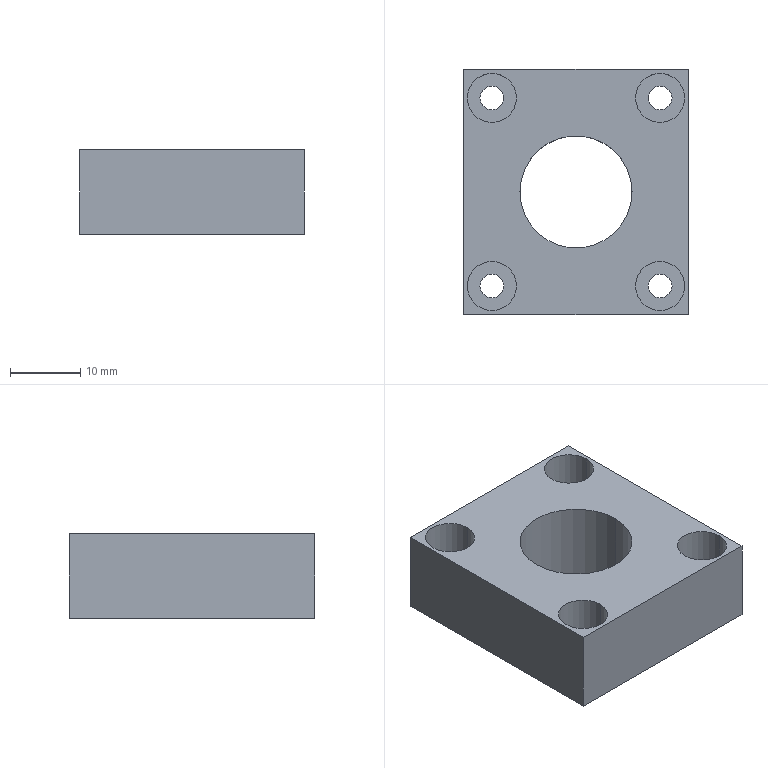Part | NX | features BREP 1 | 1 solid | 28 faces | box 32 x 35 x 12 mm | volume 10003 mm3 | cylinder 18 | plane 10 | commonest cylinder face diameters 3.4 x8 7 x8 16 x2
STEP:
#1=CARTESIAN_POINT('',(8.5,-13.416,12.));
#2=VERTEX_POINT('',#1);
#3=CARTESIAN_POINT('',(8.5,-13.416,7.));
#4=VERTEX_POINT('',#3);
#5=CARTESIAN_POINT('',(8.5,-13.416,12.));
#6=DIRECTION('',(0.,0.,1.));
#7=VECTOR('',#6,1000.);
#8=LINE('',#5,#7);
#9=EDGE_CURVE('',#2,#4,#8,.F.);
#10=ORIENTED_EDGE('',*,*,#9,.T.);
#11=CARTESIAN_POINT('',(15.5,-13.416,7.));
#12=VERTEX_POINT('',#11);
#13=CARTESIAN_POINT('',(12.,-13.416,7.));
#14=DIRECTION('',(0.,0.,1.));
#15=DIRECTION('',(1.,0.,0.));
#16=AXIS2_PLACEMENT_3D('',#13,#14,#15);
#17=CIRCLE('',#16,3.5);
#18=EDGE_CURVE('',#12,#4,#17,.T.);
#19=ORIENTED_EDGE('',*,*,#18,.F.);
#20=CARTESIAN_POINT('',(15.5,-13.416,12.));
#21=VERTEX_POINT('',#20);
#22=CARTESIAN_POINT('',(15.5,-13.416,12.));
#23=DIRECTION('',(0.,0.,1.));
#24=VECTOR('',#23,1000.);
#25=LINE('',#22,#24);
#26=EDGE_CURVE('',#21,#12,#25,.F.);
#27=ORIENTED_EDGE('',*,*,#26,.F.);
#28=CARTESIAN_POINT('',(12.,-13.416,12.));
#29=DIRECTION('',(0.,0.,1.));
#30=DIRECTION('',(1.,0.,0.));
#31=AXIS2_PLACEMENT_3D('',#28,#29,#30);
#32=CIRCLE('',#31,3.5);
#33=EDGE_CURVE('',#21,#2,#32,.T.);
#34=ORIENTED_EDGE('',*,*,#33,.T.);
#35=EDGE_LOOP('',(#10,#19,#27,#34));
#36=FACE_BOUND('',#35,.T.);
#37=CARTESIAN_POINT('',(12.,-13.416,12.));
#38=DIRECTION('',(0.,0.,1.));
#39=DIRECTION('',(1.,0.,0.));
#40=AXIS2_PLACEMENT_3D('',#37,#38,#39);
#41=CYLINDRICAL_SURFACE('',#40,3.5);
#42=ADVANCED_FACE('',(#36),#41,.F.);
#43=ORIENTED_EDGE('',*,*,#18,.T.);
#44=CARTESIAN_POINT('',(12.,-13.416,7.));
#45=DIRECTION('',(0.,0.,1.));
#46=DIRECTION('',(1.,0.,0.));
#47=AXIS2_PLACEMENT_3D('',#44,#45,#46);
#48=CIRCLE('',#47,3.5);
#49=EDGE_CURVE('',#4,#12,#48,.T.);
#50=ORIENTED_EDGE('',*,*,#49,.T.);
#51=EDGE_LOOP('',(#43,#50));
#52=FACE_BOUND('',#51,.T.);
#53=CARTESIAN_POINT('',(13.7,-13.416,7.));
#54=VERTEX_POINT('',#53);
#55=CARTESIAN_POINT('',(10.3,-13.416,7.));
#56=VERTEX_POINT('',#55);
#57=CARTESIAN_POINT('',(12.,-13.416,7.));
#58=DIRECTION('',(0.,0.,1.));
#59=DIRECTION('',(1.,0.,0.));
#60=AXIS2_PLACEMENT_3D('',#57,#58,#59);
#61=CIRCLE('',#60,1.7);
#62=EDGE_CURVE('',#54,#56,#61,.T.);
#63=ORIENTED_EDGE('',*,*,#62,.F.);
#64=CARTESIAN_POINT('',(12.,-13.416,7.));
#65=DIRECTION('',(0.,0.,1.));
#66=DIRECTION('',(1.,0.,0.));
#67=AXIS2_PLACEMENT_3D('',#64,#65,#66);
#68=CIRCLE('',#67,1.7);
#69=EDGE_CURVE('',#56,#54,#68,.T.);
#70=ORIENTED_EDGE('',*,*,#69,.F.);
#71=EDGE_LOOP('',(#63,#70));
#72=FACE_BOUND('',#71,.T.);
#73=CARTESIAN_POINT('',(13.7,-13.416,7.));
#74=DIRECTION('',(0.,0.,-1.));
#75=DIRECTION('',(-1.,0.,0.));
#76=AXIS2_PLACEMENT_3D('',#73,#74,#75);
#77=PLANE('',#76);
#78=ADVANCED_FACE('',(#52,#72),#77,.F.);
#79=CARTESIAN_POINT('',(10.3,-13.416,0.));
#80=VERTEX_POINT('',#79);
#81=CARTESIAN_POINT('',(10.3,-13.416,12.));
#82=DIRECTION('',(0.,0.,1.));
#83=VECTOR('',#82,1000.);
#84=LINE('',#81,#83);
#85=EDGE_CURVE('',#56,#80,#84,.F.);
#86=ORIENTED_EDGE('',*,*,#85,.T.);
#87=CARTESIAN_POINT('',(13.7,-13.416,0.));
#88=VERTEX_POINT('',#87);
#89=CARTESIAN_POINT('',(12.,-13.416,0.));
#90=DIRECTION('',(0.,0.,1.));
#91=DIRECTION('',(1.,0.,0.));
#92=AXIS2_PLACEMENT_3D('',#89,#90,#91);
#93=CIRCLE('',#92,1.7);
#94=EDGE_CURVE('',#88,#80,#93,.T.);
#95=ORIENTED_EDGE('',*,*,#94,.F.);
#96=CARTESIAN_POINT('',(13.7,-13.416,12.));
#97=DIRECTION('',(0.,0.,1.));
#98=VECTOR('',#97,1000.);
#99=LINE('',#96,#98);
#100=EDGE_CURVE('',#54,#88,#99,.F.);
#101=ORIENTED_EDGE('',*,*,#100,.F.);
#102=ORIENTED_EDGE('',*,*,#62,.T.);
#103=EDGE_LOOP('',(#86,#95,#101,#102));
#104=FACE_BOUND('',#103,.T.);
#105=CARTESIAN_POINT('',(12.,-13.416,12.));
#106=DIRECTION('',(0.,0.,1.));
#107=DIRECTION('',(1.,0.,0.));
#108=AXIS2_PLACEMENT_3D('',#105,#106,#107);
#109=CYLINDRICAL_SURFACE('',#108,1.7);
#110=ADVANCED_FACE('',(#104),#109,.F.);
#111=CARTESIAN_POINT('',(-15.5,-13.416,12.));
#112=VERTEX_POINT('',#111);
#113=CARTESIAN_POINT('',(-15.5,-13.416,7.));
#114=VERTEX_POINT('',#113);
#115=CARTESIAN_POINT('',(-15.5,-13.416,12.));
#116=DIRECTION('',(0.,0.,1.));
#117=VECTOR('',#116,1000.);
#118=LINE('',#115,#117);
#119=EDGE_CURVE('',#112,#114,#118,.F.);
#120=ORIENTED_EDGE('',*,*,#119,.T.);
#121=CARTESIAN_POINT('',(-8.5,-13.416,7.));
#122=VERTEX_POINT('',#121);
#123=CARTESIAN_POINT('',(-12.,-13.416,7.));
#124=DIRECTION('',(0.,0.,1.));
#125=DIRECTION('',(1.,0.,0.));
#126=AXIS2_PLACEMENT_3D('',#123,#124,#125);
#127=CIRCLE('',#126,3.5);
#128=EDGE_CURVE('',#122,#114,#127,.T.);
#129=ORIENTED_EDGE('',*,*,#128,.F.);
#130=CARTESIAN_POINT('',(-8.5,-13.416,12.));
#131=VERTEX_POINT('',#130);
#132=CARTESIAN_POINT('',(-8.5,-13.416,12.));
#133=DIRECTION('',(0.,0.,1.));
#134=VECTOR('',#133,1000.);
#135=LINE('',#132,#134);
#136=EDGE_CURVE('',#131,#122,#135,.F.);
#137=ORIENTED_EDGE('',*,*,#136,.F.);
#138=CARTESIAN_POINT('',(-12.,-13.416,12.));
#139=DIRECTION('',(0.,0.,1.));
#140=DIRECTION('',(1.,0.,0.));
#141=AXIS2_PLACEMENT_3D('',#138,#139,#140);
#142=CIRCLE('',#141,3.5);
#143=EDGE_CURVE('',#131,#112,#142,.T.);
#144=ORIENTED_EDGE('',*,*,#143,.T.);
#145=EDGE_LOOP('',(#120,#129,#137,#144));
#146=FACE_BOUND('',#145,.T.);
#147=CARTESIAN_POINT('',(-12.,-13.416,12.));
#148=DIRECTION('',(0.,0.,1.));
#149=DIRECTION('',(1.,0.,0.));
#150=AXIS2_PLACEMENT_3D('',#147,#148,#149);
#151=CYLINDRICAL_SURFACE('',#150,3.5);
#152=ADVANCED_FACE('',(#146),#151,.F.);
#153=ORIENTED_EDGE('',*,*,#128,.T.);
#154=CARTESIAN_POINT('',(-12.,-13.416,7.));
#155=DIRECTION('',(0.,0.,1.));
#156=DIRECTION('',(1.,0.,0.));
#157=AXIS2_PLACEMENT_3D('',#154,#155,#156);
#158=CIRCLE('',#157,3.5);
#159=EDGE_CURVE('',#114,#122,#158,.T.);
#160=ORIENTED_EDGE('',*,*,#159,.T.);
#161=EDGE_LOOP('',(#153,#160));
#162=FACE_BOUND('',#161,.T.);
#163=CARTESIAN_POINT('',(-10.3,-13.416,7.));
#164=VERTEX_POINT('',#163);
#165=CARTESIAN_POINT('',(-13.7,-13.416,7.));
#166=VERTEX_POINT('',#165);
#167=CARTESIAN_POINT('',(-12.,-13.416,7.));
#168=DIRECTION('',(0.,0.,1.));
#169=DIRECTION('',(1.,0.,0.));
#170=AXIS2_PLACEMENT_3D('',#167,#168,#169);
#171=CIRCLE('',#170,1.7);
#172=EDGE_CURVE('',#164,#166,#171,.T.);
#173=ORIENTED_EDGE('',*,*,#172,.F.);
#174=CARTESIAN_POINT('',(-12.,-13.416,7.));
#175=DIRECTION('',(0.,0.,1.));
#176=DIRECTION('',(1.,0.,0.));
#177=AXIS2_PLACEMENT_3D('',#174,#175,#176);
#178=CIRCLE('',#177,1.7);
#179=EDGE_CURVE('',#166,#164,#178,.T.);
#180=ORIENTED_EDGE('',*,*,#179,.F.);
#181=EDGE_LOOP('',(#173,#180));
#182=FACE_BOUND('',#181,.T.);
#183=CARTESIAN_POINT('',(-10.3,-13.416,7.));
#184=DIRECTION('',(0.,0.,-1.));
#185=DIRECTION('',(-1.,0.,0.));
#186=AXIS2_PLACEMENT_3D('',#183,#184,#185);
#187=PLANE('',#186);
#188=ADVANCED_FACE('',(#162,#182),#187,.F.);
#189=CARTESIAN_POINT('',(-13.7,-13.416,0.));
#190=VERTEX_POINT('',#189);
#191=CARTESIAN_POINT('',(-13.7,-13.416,12.));
#192=DIRECTION('',(0.,0.,1.));
#193=VECTOR('',#192,1000.);
#194=LINE('',#191,#193);
#195=EDGE_CURVE('',#166,#190,#194,.F.);
#196=ORIENTED_EDGE('',*,*,#195,.T.);
#197=CARTESIAN_POINT('',(-10.3,-13.416,0.));
#198=VERTEX_POINT('',#197);
#199=CARTESIAN_POINT('',(-12.,-13.416,0.));
#200=DIRECTION('',(0.,0.,1.));
#201=DIRECTION('',(1.,0.,0.));
#202=AXIS2_PLACEMENT_3D('',#199,#200,#201);
#203=CIRCLE('',#202,1.7);
#204=EDGE_CURVE('',#198,#190,#203,.T.);
#205=ORIENTED_EDGE('',*,*,#204,.F.);
#206=CARTESIAN_POINT('',(-10.3,-13.416,12.));
#207=DIRECTION('',(0.,0.,1.));
#208=VECTOR('',#207,1000.);
#209=LINE('',#206,#208);
#210=EDGE_CURVE('',#164,#198,#209,.F.);
#211=ORIENTED_EDGE('',*,*,#210,.F.);
#212=ORIENTED_EDGE('',*,*,#172,.T.);
#213=EDGE_LOOP('',(#196,#205,#211,#212));
#214=FACE_BOUND('',#213,.T.);
#215=CARTESIAN_POINT('',(-12.,-13.416,12.));
#216=DIRECTION('',(0.,0.,1.));
#217=DIRECTION('',(1.,0.,0.));
#218=AXIS2_PLACEMENT_3D('',#215,#216,#217);
#219=CYLINDRICAL_SURFACE('',#218,1.7);
#220=ADVANCED_FACE('',(#214),#219,.F.);
#221=CARTESIAN_POINT('',(8.5,13.416,12.));
#222=VERTEX_POINT('',#221);
#223=CARTESIAN_POINT('',(8.5,13.416,7.));
#224=VERTEX_POINT('',#223);
#225=CARTESIAN_POINT('',(8.5,13.416,12.));
#226=DIRECTION('',(0.,0.,1.));
#227=VECTOR('',#226,1000.);
#228=LINE('',#225,#227);
#229=EDGE_CURVE('',#222,#224,#228,.F.);
#230=ORIENTED_EDGE('',*,*,#229,.T.);
#231=CARTESIAN_POINT('',(15.5,13.416,7.));
#232=VERTEX_POINT('',#231);
#233=CARTESIAN_POINT('',(12.,13.416,7.));
#234=DIRECTION('',(0.,0.,1.));
#235=DIRECTION('',(1.,0.,0.));
#236=AXIS2_PLACEMENT_3D('',#233,#234,#235);
#237=CIRCLE('',#236,3.5);
#238=EDGE_CURVE('',#232,#224,#237,.T.);
#239=ORIENTED_EDGE('',*,*,#238,.F.);
#240=CARTESIAN_POINT('',(15.5,13.416,12.));
#241=VERTEX_POINT('',#240);
#242=CARTESIAN_POINT('',(15.5,13.416,12.));
#243=DIRECTION('',(0.,0.,1.));
#244=VECTOR('',#243,1000.);
#245=LINE('',#242,#244);
#246=EDGE_CURVE('',#241,#232,#245,.F.);
#247=ORIENTED_EDGE('',*,*,#246,.F.);
#248=CARTESIAN_POINT('',(12.,13.416,12.));
#249=DIRECTION('',(0.,0.,1.));
#250=DIRECTION('',(1.,0.,0.));
#251=AXIS2_PLACEMENT_3D('',#248,#249,#250);
#252=CIRCLE('',#251,3.5);
#253=EDGE_CURVE('',#241,#222,#252,.T.);
#254=ORIENTED_EDGE('',*,*,#253,.T.);
#255=EDGE_LOOP('',(#230,#239,#247,#254));
#256=FACE_BOUND('',#255,.T.);
#257=CARTESIAN_POINT('',(12.,13.416,12.));
#258=DIRECTION('',(0.,0.,1.));
#259=DIRECTION('',(1.,0.,0.));
#260=AXIS2_PLACEMENT_3D('',#257,#258,#259);
#261=CYLINDRICAL_SURFACE('',#260,3.5);
#262=ADVANCED_FACE('',(#256),#261,.F.);
#263=ORIENTED_EDGE('',*,*,#238,.T.);
#264=CARTESIAN_POINT('',(12.,13.416,7.));
#265=DIRECTION('',(0.,0.,1.));
#266=DIRECTION('',(1.,0.,0.));
#267=AXIS2_PLACEMENT_3D('',#264,#265,#266);
#268=CIRCLE('',#267,3.5);
#269=EDGE_CURVE('',#224,#232,#268,.T.);
#270=ORIENTED_EDGE('',*,*,#269,.T.);
#271=EDGE_LOOP('',(#263,#270));
#272=FACE_BOUND('',#271,.T.);
#273=CARTESIAN_POINT('',(13.7,13.416,7.));
#274=VERTEX_POINT('',#273);
#275=CARTESIAN_POINT('',(10.3,13.416,7.));
#276=VERTEX_POINT('',#275);
#277=CARTESIAN_POINT('',(12.,13.416,7.));
#278=DIRECTION('',(0.,0.,1.));
#279=DIRECTION('',(1.,0.,0.));
#280=AXIS2_PLACEMENT_3D('',#277,#278,#279);
#281=CIRCLE('',#280,1.7);
#282=EDGE_CURVE('',#274,#276,#281,.T.);
#283=ORIENTED_EDGE('',*,*,#282,.F.);
#284=CARTESIAN_POINT('',(12.,13.416,7.));
#285=DIRECTION('',(0.,0.,1.));
#286=DIRECTION('',(1.,0.,0.));
#287=AXIS2_PLACEMENT_3D('',#284,#285,#286);
#288=CIRCLE('',#287,1.7);
#289=EDGE_CURVE('',#276,#274,#288,.T.);
#290=ORIENTED_EDGE('',*,*,#289,.F.);
#291=EDGE_LOOP('',(#283,#290));
#292=FACE_BOUND('',#291,.T.);
#293=CARTESIAN_POINT('',(13.7,13.416,7.));
#294=DIRECTION('',(0.,0.,-1.));
#295=DIRECTION('',(-1.,0.,0.));
#296=AXIS2_PLACEMENT_3D('',#293,#294,#295);
#297=PLANE('',#296);
#298=ADVANCED_FACE('',(#272,#292),#297,.F.);
#299=CARTESIAN_POINT('',(10.3,13.416,0.));
#300=VERTEX_POINT('',#299);
#301=CARTESIAN_POINT('',(10.3,13.416,12.));
#302=DIRECTION('',(0.,0.,1.));
#303=VECTOR('',#302,1000.);
#304=LINE('',#301,#303);
#305=EDGE_CURVE('',#276,#300,#304,.F.);
#306=ORIENTED_EDGE('',*,*,#305,.T.);
#307=CARTESIAN_POINT('',(13.7,13.416,0.));
#308=VERTEX_POINT('',#307);
#309=CARTESIAN_POINT('',(12.,13.416,0.));
#310=DIRECTION('',(0.,0.,1.));
#311=DIRECTION('',(1.,0.,0.));
#312=AXIS2_PLACEMENT_3D('',#309,#310,#311);
#313=CIRCLE('',#312,1.7);
#314=EDGE_CURVE('',#308,#300,#313,.T.);
#315=ORIENTED_EDGE('',*,*,#314,.F.);
#316=CARTESIAN_POINT('',(13.7,13.416,12.));
#317=DIRECTION('',(0.,0.,1.));
#318=VECTOR('',#317,1000.);
#319=LINE('',#316,#318);
#320=EDGE_CURVE('',#274,#308,#319,.F.);
#321=ORIENTED_EDGE('',*,*,#320,.F.);
#322=ORIENTED_EDGE('',*,*,#282,.T.);
#323=EDGE_LOOP('',(#306,#315,#321,#322));
#324=FACE_BOUND('',#323,.T.);
#325=CARTESIAN_POINT('',(12.,13.416,12.));
#326=DIRECTION('',(0.,0.,1.));
#327=DIRECTION('',(1.,0.,0.));
#328=AXIS2_PLACEMENT_3D('',#325,#326,#327);
#329=CYLINDRICAL_SURFACE('',#328,1.7);
#330=ADVANCED_FACE('',(#324),#329,.F.);
#331=CARTESIAN_POINT('',(-15.5,13.416,12.));
#332=VERTEX_POINT('',#331);
#333=CARTESIAN_POINT('',(-15.5,13.416,7.));
#334=VERTEX_POINT('',#333);
#335=CARTESIAN_POINT('',(-15.5,13.416,12.));
#336=DIRECTION('',(0.,0.,1.));
#337=VECTOR('',#336,1000.);
#338=LINE('',#335,#337);
#339=EDGE_CURVE('',#332,#334,#338,.F.);
#340=ORIENTED_EDGE('',*,*,#339,.T.);
#341=CARTESIAN_POINT('',(-8.5,13.416,7.));
#342=VERTEX_POINT('',#341);
#343=CARTESIAN_POINT('',(-12.,13.416,7.));
#344=DIRECTION('',(0.,0.,1.));
#345=DIRECTION('',(1.,0.,0.));
#346=AXIS2_PLACEMENT_3D('',#343,#344,#345);
#347=CIRCLE('',#346,3.5);
#348=EDGE_CURVE('',#342,#334,#347,.T.);
#349=ORIENTED_EDGE('',*,*,#348,.F.);
#350=CARTESIAN_POINT('',(-8.5,13.416,12.));
#351=VERTEX_POINT('',#350);
#352=CARTESIAN_POINT('',(-8.5,13.416,12.));
#353=DIRECTION('',(0.,0.,1.));
#354=VECTOR('',#353,1000.);
#355=LINE('',#352,#354);
#356=EDGE_CURVE('',#351,#342,#355,.F.);
#357=ORIENTED_EDGE('',*,*,#356,.F.);
#358=CARTESIAN_POINT('',(-12.,13.416,12.));
#359=DIRECTION('',(0.,0.,1.));
#360=DIRECTION('',(1.,0.,0.));
#361=AXIS2_PLACEMENT_3D('',#358,#359,#360);
#362=CIRCLE('',#361,3.5);
#363=EDGE_CURVE('',#351,#332,#362,.T.);
#364=ORIENTED_EDGE('',*,*,#363,.T.);
#365=EDGE_LOOP('',(#340,#349,#357,#364));
#366=FACE_BOUND('',#365,.T.);
#367=CARTESIAN_POINT('',(-12.,13.416,12.));
#368=DIRECTION('',(0.,0.,1.));
#369=DIRECTION('',(1.,0.,0.));
#370=AXIS2_PLACEMENT_3D('',#367,#368,#369);
#371=CYLINDRICAL_SURFACE('',#370,3.5);
#372=ADVANCED_FACE('',(#366),#371,.F.);
#373=ORIENTED_EDGE('',*,*,#348,.T.);
#374=CARTESIAN_POINT('',(-12.,13.416,7.));
#375=DIRECTION('',(0.,0.,1.));
#376=DIRECTION('',(1.,0.,0.));
#377=AXIS2_PLACEMENT_3D('',#374,#375,#376);
#378=CIRCLE('',#377,3.5);
#379=EDGE_CURVE('',#334,#342,#378,.T.);
#380=ORIENTED_EDGE('',*,*,#379,.T.);
#381=EDGE_LOOP('',(#373,#380));
#382=FACE_BOUND('',#381,.T.);
#383=CARTESIAN_POINT('',(-10.3,13.416,7.));
#384=VERTEX_POINT('',#383);
#385=CARTESIAN_POINT('',(-13.7,13.416,7.));
#386=VERTEX_POINT('',#385);
#387=CARTESIAN_POINT('',(-12.,13.416,7.));
#388=DIRECTION('',(0.,0.,1.));
#389=DIRECTION('',(1.,0.,0.));
#390=AXIS2_PLACEMENT_3D('',#387,#388,#389);
#391=CIRCLE('',#390,1.7);
#392=EDGE_CURVE('',#384,#386,#391,.T.);
#393=ORIENTED_EDGE('',*,*,#392,.F.);
#394=CARTESIAN_POINT('',(-12.,13.416,7.));
#395=DIRECTION('',(0.,0.,1.));
#396=DIRECTION('',(1.,0.,0.));
#397=AXIS2_PLACEMENT_3D('',#394,#395,#396);
#398=CIRCLE('',#397,1.7);
#399=EDGE_CURVE('',#386,#384,#398,.T.);
#400=ORIENTED_EDGE('',*,*,#399,.F.);
#401=EDGE_LOOP('',(#393,#400));
#402=FACE_BOUND('',#401,.T.);
#403=CARTESIAN_POINT('',(-10.3,13.416,7.));
#404=DIRECTION('',(0.,0.,-1.));
#405=DIRECTION('',(-1.,0.,0.));
#406=AXIS2_PLACEMENT_3D('',#403,#404,#405);
#407=PLANE('',#406);
#408=ADVANCED_FACE('',(#382,#402),#407,.F.);
#409=CARTESIAN_POINT('',(-13.7,13.416,0.));
#410=VERTEX_POINT('',#409);
#411=CARTESIAN_POINT('',(-13.7,13.416,12.));
#412=DIRECTION('',(0.,0.,1.));
#413=VECTOR('',#412,1000.);
#414=LINE('',#411,#413);
#415=EDGE_CURVE('',#386,#410,#414,.F.);
#416=ORIENTED_EDGE('',*,*,#415,.T.);
#417=CARTESIAN_POINT('',(-10.3,13.416,0.));
#418=VERTEX_POINT('',#417);
#419=CARTESIAN_POINT('',(-12.,13.416,0.));
#420=DIRECTION('',(0.,0.,1.));
#421=DIRECTION('',(1.,0.,0.));
#422=AXIS2_PLACEMENT_3D('',#419,#420,#421);
#423=CIRCLE('',#422,1.7);
#424=EDGE_CURVE('',#418,#410,#423,.T.);
#425=ORIENTED_EDGE('',*,*,#424,.F.);
#426=CARTESIAN_POINT('',(-10.3,13.416,12.));
#427=DIRECTION('',(0.,0.,1.));
#428=VECTOR('',#427,1000.);
#429=LINE('',#426,#428);
#430=EDGE_CURVE('',#384,#418,#429,.F.);
#431=ORIENTED_EDGE('',*,*,#430,.F.);
#432=ORIENTED_EDGE('',*,*,#392,.T.);
#433=EDGE_LOOP('',(#416,#425,#431,#432));
#434=FACE_BOUND('',#433,.T.);
#435=CARTESIAN_POINT('',(-12.,13.416,12.));
#436=DIRECTION('',(0.,0.,1.));
#437=DIRECTION('',(1.,0.,0.));
#438=AXIS2_PLACEMENT_3D('',#435,#436,#437);
#439=CYLINDRICAL_SURFACE('',#438,1.7);
#440=ADVANCED_FACE('',(#434),#439,.F.);
#441=CARTESIAN_POINT('',(8.,0.,12.));
#442=VERTEX_POINT('',#441);
#443=CARTESIAN_POINT('',(8.,0.,0.));
#444=VERTEX_POINT('',#443);
#445=CARTESIAN_POINT('',(8.,0.,12.));
#446=DIRECTION('',(0.,0.,-1.));
#447=VECTOR('',#446,1000.);
#448=LINE('',#445,#447);
#449=EDGE_CURVE('',#442,#444,#448,.T.);
#450=ORIENTED_EDGE('',*,*,#449,.F.);
#451=CARTESIAN_POINT('',(-8.,0.,12.));
#452=VERTEX_POINT('',#451);
#453=CARTESIAN_POINT('',(0.,0.,12.));
#454=DIRECTION('',(0.,0.,1.));
#455=DIRECTION('',(1.,0.,0.));
#456=AXIS2_PLACEMENT_3D('',#453,#454,#455);
#457=CIRCLE('',#456,8.);
#458=EDGE_CURVE('',#442,#452,#457,.T.);
#459=ORIENTED_EDGE('',*,*,#458,.T.);
#460=CARTESIAN_POINT('',(-8.,0.,0.));
#461=VERTEX_POINT('',#460);
#462=CARTESIAN_POINT('',(-8.,0.,12.));
#463=DIRECTION('',(0.,0.,-1.));
#464=VECTOR('',#463,1000.);
#465=LINE('',#462,#464);
#466=EDGE_CURVE('',#452,#461,#465,.T.);
#467=ORIENTED_EDGE('',*,*,#466,.T.);
#468=CARTESIAN_POINT('',(0.,0.,0.));
#469=DIRECTION('',(0.,0.,1.));
#470=DIRECTION('',(1.,0.,0.));
#471=AXIS2_PLACEMENT_3D('',#468,#469,#470);
#472=CIRCLE('',#471,8.);
#473=EDGE_CURVE('',#444,#461,#472,.T.);
#474=ORIENTED_EDGE('',*,*,#473,.F.);
#475=EDGE_LOOP('',(#450,#459,#467,#474));
#476=FACE_BOUND('',#475,.T.);
#477=CARTESIAN_POINT('',(0.,0.,12.));
#478=DIRECTION('',(0.,0.,-1.));
#479=DIRECTION('',(-1.,0.,0.));
#480=AXIS2_PLACEMENT_3D('',#477,#478,#479);
#481=CYLINDRICAL_SURFACE('',#480,8.);
#482=ADVANCED_FACE('',(#476),#481,.F.);
#483=CARTESIAN_POINT('',(-16.,-17.5,0.));
#484=VERTEX_POINT('',#483);
#485=CARTESIAN_POINT('',(16.,-17.5,0.));
#486=VERTEX_POINT('',#485);
#487=CARTESIAN_POINT('',(-16.,-17.5,0.));
#488=DIRECTION('',(1.,0.,0.));
#489=VECTOR('',#488,1000.);
#490=LINE('',#487,#489);
#491=EDGE_CURVE('',#484,#486,#490,.T.);
#492=ORIENTED_EDGE('',*,*,#491,.T.);
#493=CARTESIAN_POINT('',(16.,-17.5,12.));
#494=VERTEX_POINT('',#493);
#495=CARTESIAN_POINT('',(16.,-17.5,12.));
#496=DIRECTION('',(0.,0.,-1.));
#497=VECTOR('',#496,1000.);
#498=LINE('',#495,#497);
#499=EDGE_CURVE('',#494,#486,#498,.T.);
#500=ORIENTED_EDGE('',*,*,#499,.F.);
#501=CARTESIAN_POINT('',(-16.,-17.5,12.));
#502=VERTEX_POINT('',#501);
#503=CARTESIAN_POINT('',(-16.,-17.5,12.));
#504=DIRECTION('',(1.,0.,0.));
#505=VECTOR('',#504,1000.);
#506=LINE('',#503,#505);
#507=EDGE_CURVE('',#502,#494,#506,.T.);
#508=ORIENTED_EDGE('',*,*,#507,.F.);
#509=CARTESIAN_POINT('',(-16.,-17.5,12.));
#510=DIRECTION('',(0.,0.,-1.));
#511=VECTOR('',#510,1000.);
#512=LINE('',#509,#511);
#513=EDGE_CURVE('',#502,#484,#512,.T.);
#514=ORIENTED_EDGE('',*,*,#513,.T.);
#515=EDGE_LOOP('',(#492,#500,#508,#514));
#516=FACE_BOUND('',#515,.T.);
#517=CARTESIAN_POINT('',(-16.,-17.5,12.));
#518=DIRECTION('',(0.,1.,0.));
#519=DIRECTION('',(0.,0.,1.));
#520=AXIS2_PLACEMENT_3D('',#517,#518,#519);
#521=PLANE('',#520);
#522=ADVANCED_FACE('',(#516),#521,.F.);
#523=CARTESIAN_POINT('',(-16.,17.5,0.));
#524=VERTEX_POINT('',#523);
#525=CARTESIAN_POINT('',(-16.,-17.5,0.));
#526=DIRECTION('',(0.,-1.,0.));
#527=VECTOR('',#526,1000.);
#528=LINE('',#525,#527);
#529=EDGE_CURVE('',#524,#484,#528,.T.);
#530=ORIENTED_EDGE('',*,*,#529,.T.);
#531=ORIENTED_EDGE('',*,*,#513,.F.);
#532=CARTESIAN_POINT('',(-16.,17.5,12.));
#533=VERTEX_POINT('',#532);
#534=CARTESIAN_POINT('',(-16.,-17.5,12.));
#535=DIRECTION('',(0.,-1.,0.));
#536=VECTOR('',#535,1000.);
#537=LINE('',#534,#536);
#538=EDGE_CURVE('',#533,#502,#537,.T.);
#539=ORIENTED_EDGE('',*,*,#538,.F.);
#540=CARTESIAN_POINT('',(-16.,17.5,12.));
#541=DIRECTION('',(0.,0.,-1.));
#542=VECTOR('',#541,1000.);
#543=LINE('',#540,#542);
#544=EDGE_CURVE('',#533,#524,#543,.T.);
#545=ORIENTED_EDGE('',*,*,#544,.T.);
#546=EDGE_LOOP('',(#530,#531,#539,#545));
#547=FACE_BOUND('',#546,.T.);
#548=CARTESIAN_POINT('',(-16.,-17.5,12.));
#549=DIRECTION('',(1.,0.,0.));
#550=DIRECTION('',(0.,0.,-1.));
#551=AXIS2_PLACEMENT_3D('',#548,#549,#550);
#552=PLANE('',#551);
#553=ADVANCED_FACE('',(#547),#552,.F.);
#554=CARTESIAN_POINT('',(16.,17.5,0.));
#555=VERTEX_POINT('',#554);
#556=CARTESIAN_POINT('',(-16.,17.5,0.));
#557=DIRECTION('',(-1.,0.,0.));
#558=VECTOR('',#557,1000.);
#559=LINE('',#556,#558);
#560=EDGE_CURVE('',#555,#524,#559,.T.);
#561=ORIENTED_EDGE('',*,*,#560,.T.);
#562=ORIENTED_EDGE('',*,*,#544,.F.);
#563=CARTESIAN_POINT('',(16.,17.5,12.));
#564=VERTEX_POINT('',#563);
#565=CARTESIAN_POINT('',(-16.,17.5,12.));
#566=DIRECTION('',(-1.,0.,0.));
#567=VECTOR('',#566,1000.);
#568=LINE('',#565,#567);
#569=EDGE_CURVE('',#564,#533,#568,.T.);
#570=ORIENTED_EDGE('',*,*,#569,.F.);
#571=CARTESIAN_POINT('',(16.,17.5,12.));
#572=DIRECTION('',(0.,0.,-1.));
#573=VECTOR('',#572,1000.);
#574=LINE('',#571,#573);
#575=EDGE_CURVE('',#564,#555,#574,.T.);
#576=ORIENTED_EDGE('',*,*,#575,.T.);
#577=EDGE_LOOP('',(#561,#562,#570,#576));
#578=FACE_BOUND('',#577,.T.);
#579=CARTESIAN_POINT('',(-16.,17.5,12.));
#580=DIRECTION('',(0.,-1.,0.));
#581=DIRECTION('',(0.,0.,-1.));
#582=AXIS2_PLACEMENT_3D('',#579,#580,#581);
#583=PLANE('',#582);
#584=ADVANCED_FACE('',(#578),#583,.F.);
#585=CARTESIAN_POINT('',(16.,-17.5,0.));
#586=DIRECTION('',(0.,1.,0.));
#587=VECTOR('',#586,1000.);
#588=LINE('',#585,#587);
#589=EDGE_CURVE('',#486,#555,#588,.T.);
#590=ORIENTED_EDGE('',*,*,#589,.T.);
#591=ORIENTED_EDGE('',*,*,#575,.F.);
#592=CARTESIAN_POINT('',(16.,-17.5,12.));
#593=DIRECTION('',(0.,1.,0.));
#594=VECTOR('',#593,1000.);
#595=LINE('',#592,#594);
#596=EDGE_CURVE('',#494,#564,#595,.T.);
#597=ORIENTED_EDGE('',*,*,#596,.F.);
#598=ORIENTED_EDGE('',*,*,#499,.T.);
#599=EDGE_LOOP('',(#590,#591,#597,#598));
#600=FACE_BOUND('',#599,.T.);
#601=CARTESIAN_POINT('',(16.,-17.5,12.));
#602=DIRECTION('',(-1.,0.,0.));
#603=DIRECTION('',(0.,0.,1.));
#604=AXIS2_PLACEMENT_3D('',#601,#602,#603);
#605=PLANE('',#604);
#606=ADVANCED_FACE('',(#600),#605,.F.);
#607=CARTESIAN_POINT('',(0.,0.,0.));
#608=DIRECTION('',(0.,0.,1.));
#609=DIRECTION('',(1.,0.,0.));
#610=AXIS2_PLACEMENT_3D('',#607,#608,#609);
#611=CIRCLE('',#610,8.);
#612=EDGE_CURVE('',#461,#444,#611,.T.);
#613=ORIENTED_EDGE('',*,*,#612,.T.);
#614=ORIENTED_EDGE('',*,*,#473,.T.);
#615=EDGE_LOOP('',(#613,#614));
#616=FACE_BOUND('',#615,.T.);
#617=ORIENTED_EDGE('',*,*,#589,.F.);
#618=ORIENTED_EDGE('',*,*,#491,.F.);
#619=ORIENTED_EDGE('',*,*,#529,.F.);
#620=ORIENTED_EDGE('',*,*,#560,.F.);
#621=EDGE_LOOP('',(#617,#618,#619,#620));
#622=FACE_BOUND('',#621,.T.);
#623=ORIENTED_EDGE('',*,*,#424,.T.);
#624=CARTESIAN_POINT('',(-12.,13.416,0.));
#625=DIRECTION('',(0.,0.,1.));
#626=DIRECTION('',(1.,0.,0.));
#627=AXIS2_PLACEMENT_3D('',#624,#625,#626);
#628=CIRCLE('',#627,1.7);
#629=EDGE_CURVE('',#410,#418,#628,.T.);
#630=ORIENTED_EDGE('',*,*,#629,.T.);
#631=EDGE_LOOP('',(#623,#630));
#632=FACE_BOUND('',#631,.T.);
#633=ORIENTED_EDGE('',*,*,#314,.T.);
#634=CARTESIAN_POINT('',(12.,13.416,0.));
#635=DIRECTION('',(0.,0.,1.));
#636=DIRECTION('',(1.,0.,0.));
#637=AXIS2_PLACEMENT_3D('',#634,#635,#636);
#638=CIRCLE('',#637,1.7);
#639=EDGE_CURVE('',#300,#308,#638,.T.);
#640=ORIENTED_EDGE('',*,*,#639,.T.);
#641=EDGE_LOOP('',(#633,#640));
#642=FACE_BOUND('',#641,.T.);
#643=ORIENTED_EDGE('',*,*,#204,.T.);
#644=CARTESIAN_POINT('',(-12.,-13.416,0.));
#645=DIRECTION('',(0.,0.,1.));
#646=DIRECTION('',(1.,0.,0.));
#647=AXIS2_PLACEMENT_3D('',#644,#645,#646);
#648=CIRCLE('',#647,1.7);
#649=EDGE_CURVE('',#190,#198,#648,.T.);
#650=ORIENTED_EDGE('',*,*,#649,.T.);
#651=EDGE_LOOP('',(#643,#650));
#652=FACE_BOUND('',#651,.T.);
#653=ORIENTED_EDGE('',*,*,#94,.T.);
#654=CARTESIAN_POINT('',(12.,-13.416,0.));
#655=DIRECTION('',(0.,0.,1.));
#656=DIRECTION('',(1.,0.,0.));
#657=AXIS2_PLACEMENT_3D('',#654,#655,#656);
#658=CIRCLE('',#657,1.7);
#659=EDGE_CURVE('',#80,#88,#658,.T.);
#660=ORIENTED_EDGE('',*,*,#659,.T.);
#661=EDGE_LOOP('',(#653,#660));
#662=FACE_BOUND('',#661,.T.);
#663=CARTESIAN_POINT('',(0.,0.,0.));
#664=DIRECTION('',(0.,0.,-1.));
#665=DIRECTION('',(-1.,0.,0.));
#666=AXIS2_PLACEMENT_3D('',#663,#664,#665);
#667=PLANE('',#666);
#668=ADVANCED_FACE('',(#616,#622,#632,#642,#652,#662),#667,.T.);
#669=CARTESIAN_POINT('',(0.,0.,12.));
#670=DIRECTION('',(0.,0.,1.));
#671=DIRECTION('',(1.,0.,0.));
#672=AXIS2_PLACEMENT_3D('',#669,#670,#671);
#673=CIRCLE('',#672,8.);
#674=EDGE_CURVE('',#452,#442,#673,.T.);
#675=ORIENTED_EDGE('',*,*,#674,.F.);
#676=ORIENTED_EDGE('',*,*,#458,.F.);
#677=EDGE_LOOP('',(#675,#676));
#678=FACE_BOUND('',#677,.T.);
#679=ORIENTED_EDGE('',*,*,#596,.T.);
#680=ORIENTED_EDGE('',*,*,#569,.T.);
#681=ORIENTED_EDGE('',*,*,#538,.T.);
#682=ORIENTED_EDGE('',*,*,#507,.T.);
#683=EDGE_LOOP('',(#679,#680,#681,#682));
#684=FACE_BOUND('',#683,.T.);
#685=ORIENTED_EDGE('',*,*,#363,.F.);
#686=CARTESIAN_POINT('',(-12.,13.416,12.));
#687=DIRECTION('',(0.,0.,1.));
#688=DIRECTION('',(1.,0.,0.));
#689=AXIS2_PLACEMENT_3D('',#686,#687,#688);
#690=CIRCLE('',#689,3.5);
#691=EDGE_CURVE('',#332,#351,#690,.T.);
#692=ORIENTED_EDGE('',*,*,#691,.F.);
#693=EDGE_LOOP('',(#685,#692));
#694=FACE_BOUND('',#693,.T.);
#695=ORIENTED_EDGE('',*,*,#253,.F.);
#696=CARTESIAN_POINT('',(12.,13.416,12.));
#697=DIRECTION('',(0.,0.,1.));
#698=DIRECTION('',(1.,0.,0.));
#699=AXIS2_PLACEMENT_3D('',#696,#697,#698);
#700=CIRCLE('',#699,3.5);
#701=EDGE_CURVE('',#222,#241,#700,.T.);
#702=ORIENTED_EDGE('',*,*,#701,.F.);
#703=EDGE_LOOP('',(#695,#702));
#704=FACE_BOUND('',#703,.T.);
#705=ORIENTED_EDGE('',*,*,#143,.F.);
#706=CARTESIAN_POINT('',(-12.,-13.416,12.));
#707=DIRECTION('',(0.,0.,1.));
#708=DIRECTION('',(1.,0.,0.));
#709=AXIS2_PLACEMENT_3D('',#706,#707,#708);
#710=CIRCLE('',#709,3.5);
#711=EDGE_CURVE('',#112,#131,#710,.T.);
#712=ORIENTED_EDGE('',*,*,#711,.F.);
#713=EDGE_LOOP('',(#705,#712));
#714=FACE_BOUND('',#713,.T.);
#715=ORIENTED_EDGE('',*,*,#33,.F.);
#716=CARTESIAN_POINT('',(12.,-13.416,12.));
#717=DIRECTION('',(0.,0.,1.));
#718=DIRECTION('',(1.,0.,0.));
#719=AXIS2_PLACEMENT_3D('',#716,#717,#718);
#720=CIRCLE('',#719,3.5);
#721=EDGE_CURVE('',#2,#21,#720,.T.);
#722=ORIENTED_EDGE('',*,*,#721,.F.);
#723=EDGE_LOOP('',(#715,#722));
#724=FACE_BOUND('',#723,.T.);
#725=CARTESIAN_POINT('',(0.,0.,12.));
#726=DIRECTION('',(0.,0.,-1.));
#727=DIRECTION('',(-1.,0.,0.));
#728=AXIS2_PLACEMENT_3D('',#725,#726,#727);
#729=PLANE('',#728);
#730=ADVANCED_FACE('',(#678,#684,#694,#704,#714,#724),#729,.F.);
#731=ORIENTED_EDGE('',*,*,#674,.T.);
#732=ORIENTED_EDGE('',*,*,#449,.T.);
#733=ORIENTED_EDGE('',*,*,#612,.F.);
#734=ORIENTED_EDGE('',*,*,#466,.F.);
#735=EDGE_LOOP('',(#731,#732,#733,#734));
#736=FACE_BOUND('',#735,.T.);
#737=CARTESIAN_POINT('',(0.,0.,12.));
#738=DIRECTION('',(0.,0.,-1.));
#739=DIRECTION('',(-1.,0.,0.));
#740=AXIS2_PLACEMENT_3D('',#737,#738,#739);
#741=CYLINDRICAL_SURFACE('',#740,8.);
#742=ADVANCED_FACE('',(#736),#741,.F.);
#743=ORIENTED_EDGE('',*,*,#629,.F.);
#744=ORIENTED_EDGE('',*,*,#415,.F.);
#745=ORIENTED_EDGE('',*,*,#399,.T.);
#746=ORIENTED_EDGE('',*,*,#430,.T.);
#747=EDGE_LOOP('',(#743,#744,#745,#746));
#748=FACE_BOUND('',#747,.T.);
#749=CARTESIAN_POINT('',(-12.,13.416,12.));
#750=DIRECTION('',(0.,0.,1.));
#751=DIRECTION('',(1.,0.,0.));
#752=AXIS2_PLACEMENT_3D('',#749,#750,#751);
#753=CYLINDRICAL_SURFACE('',#752,1.7);
#754=ADVANCED_FACE('',(#748),#753,.F.);
#755=ORIENTED_EDGE('',*,*,#379,.F.);
#756=ORIENTED_EDGE('',*,*,#339,.F.);
#757=ORIENTED_EDGE('',*,*,#691,.T.);
#758=ORIENTED_EDGE('',*,*,#356,.T.);
#759=EDGE_LOOP('',(#755,#756,#757,#758));
#760=FACE_BOUND('',#759,.T.);
#761=CARTESIAN_POINT('',(-12.,13.416,12.));
#762=DIRECTION('',(0.,0.,1.));
#763=DIRECTION('',(1.,0.,0.));
#764=AXIS2_PLACEMENT_3D('',#761,#762,#763);
#765=CYLINDRICAL_SURFACE('',#764,3.5);
#766=ADVANCED_FACE('',(#760),#765,.F.);
#767=ORIENTED_EDGE('',*,*,#639,.F.);
#768=ORIENTED_EDGE('',*,*,#305,.F.);
#769=ORIENTED_EDGE('',*,*,#289,.T.);
#770=ORIENTED_EDGE('',*,*,#320,.T.);
#771=EDGE_LOOP('',(#767,#768,#769,#770));
#772=FACE_BOUND('',#771,.T.);
#773=CARTESIAN_POINT('',(12.,13.416,12.));
#774=DIRECTION('',(0.,0.,1.));
#775=DIRECTION('',(1.,0.,0.));
#776=AXIS2_PLACEMENT_3D('',#773,#774,#775);
#777=CYLINDRICAL_SURFACE('',#776,1.7);
#778=ADVANCED_FACE('',(#772),#777,.F.);
#779=ORIENTED_EDGE('',*,*,#269,.F.);
#780=ORIENTED_EDGE('',*,*,#229,.F.);
#781=ORIENTED_EDGE('',*,*,#701,.T.);
#782=ORIENTED_EDGE('',*,*,#246,.T.);
#783=EDGE_LOOP('',(#779,#780,#781,#782));
#784=FACE_BOUND('',#783,.T.);
#785=CARTESIAN_POINT('',(12.,13.416,12.));
#786=DIRECTION('',(0.,0.,1.));
#787=DIRECTION('',(1.,0.,0.));
#788=AXIS2_PLACEMENT_3D('',#785,#786,#787);
#789=CYLINDRICAL_SURFACE('',#788,3.5);
#790=ADVANCED_FACE('',(#784),#789,.F.);
#791=ORIENTED_EDGE('',*,*,#649,.F.);
#792=ORIENTED_EDGE('',*,*,#195,.F.);
#793=ORIENTED_EDGE('',*,*,#179,.T.);
#794=ORIENTED_EDGE('',*,*,#210,.T.);
#795=EDGE_LOOP('',(#791,#792,#793,#794));
#796=FACE_BOUND('',#795,.T.);
#797=CARTESIAN_POINT('',(-12.,-13.416,12.));
#798=DIRECTION('',(0.,0.,1.));
#799=DIRECTION('',(1.,0.,0.));
#800=AXIS2_PLACEMENT_3D('',#797,#798,#799);
#801=CYLINDRICAL_SURFACE('',#800,1.7);
#802=ADVANCED_FACE('',(#796),#801,.F.);
#803=ORIENTED_EDGE('',*,*,#159,.F.);
#804=ORIENTED_EDGE('',*,*,#119,.F.);
#805=ORIENTED_EDGE('',*,*,#711,.T.);
#806=ORIENTED_EDGE('',*,*,#136,.T.);
#807=EDGE_LOOP('',(#803,#804,#805,#806));
#808=FACE_BOUND('',#807,.T.);
#809=CARTESIAN_POINT('',(-12.,-13.416,12.));
#810=DIRECTION('',(0.,0.,1.));
#811=DIRECTION('',(1.,0.,0.));
#812=AXIS2_PLACEMENT_3D('',#809,#810,#811);
#813=CYLINDRICAL_SURFACE('',#812,3.5);
#814=ADVANCED_FACE('',(#808),#813,.F.);
#815=ORIENTED_EDGE('',*,*,#659,.F.);
#816=ORIENTED_EDGE('',*,*,#85,.F.);
#817=ORIENTED_EDGE('',*,*,#69,.T.);
#818=ORIENTED_EDGE('',*,*,#100,.T.);
#819=EDGE_LOOP('',(#815,#816,#817,#818));
#820=FACE_BOUND('',#819,.T.);
#821=CARTESIAN_POINT('',(12.,-13.416,12.));
#822=DIRECTION('',(0.,0.,1.));
#823=DIRECTION('',(1.,0.,0.));
#824=AXIS2_PLACEMENT_3D('',#821,#822,#823);
#825=CYLINDRICAL_SURFACE('',#824,1.7);
#826=ADVANCED_FACE('',(#820),#825,.F.);
#827=ORIENTED_EDGE('',*,*,#49,.F.);
#828=ORIENTED_EDGE('',*,*,#9,.F.);
#829=ORIENTED_EDGE('',*,*,#721,.T.);
#830=ORIENTED_EDGE('',*,*,#26,.T.);
#831=EDGE_LOOP('',(#827,#828,#829,#830));
#832=FACE_BOUND('',#831,.T.);
#833=CARTESIAN_POINT('',(12.,-13.416,12.));
#834=DIRECTION('',(0.,0.,1.));
#835=DIRECTION('',(1.,0.,0.));
#836=AXIS2_PLACEMENT_3D('',#833,#834,#835);
#837=CYLINDRICAL_SURFACE('',#836,3.5);
#838=ADVANCED_FACE('',(#832),#837,.F.);
#839=CLOSED_SHELL('',(#42,#78,#110,#152,#188,#220,#262,#298,#330,#372,#408,#440,#482,#522,#553,#584,#606,#668,#730,#742,#754,#766,#778,#790,#802,#814,#826,#838));
#840=MANIFOLD_SOLID_BREP('',#839);
#841=(LENGTH_UNIT()NAMED_UNIT(*)SI_UNIT(.MILLI.,.METRE.));
#842=UNCERTAINTY_MEASURE_WITH_UNIT(LENGTH_MEASURE(0.00001),#841,'','');
#843=(NAMED_UNIT(*)PLANE_ANGLE_UNIT()SI_UNIT($,.RADIAN.));
#844=(NAMED_UNIT(*)SI_UNIT($,.STERADIAN.)SOLID_ANGLE_UNIT());
#845=(GEOMETRIC_REPRESENTATION_CONTEXT(3)GLOBAL_UNCERTAINTY_ASSIGNED_CONTEXT((#842))GLOBAL_UNIT_ASSIGNED_CONTEXT((#841,#843,#844))REPRESENTATION_CONTEXT('',''));
#846=ADVANCED_BREP_SHAPE_REPRESENTATION('',(#840),#845);